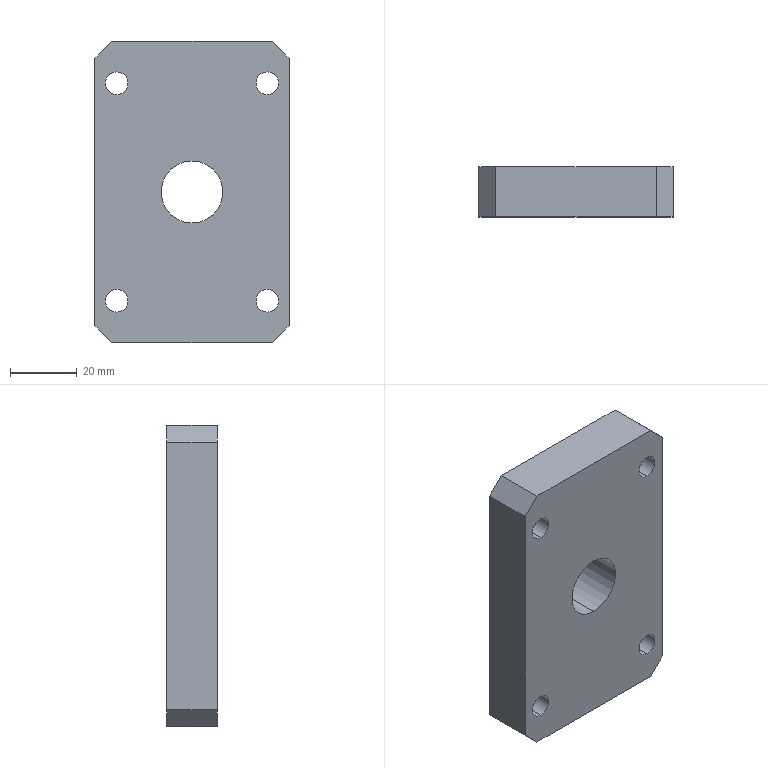Part | SolidWorks | features HoleWzd 2, Chamfer 1, Extrusion 1 | 1 solid | 20 faces | box 58 x 15 x 90 mm | volume 71339 mm3 | cylinder 10 | plane 10 | commonest cylinder face diameters 6.8 x8 18.5 x2
STEP:
#1=CARTESIAN_POINT('',(0.,-7.5,-9.25));
#2=VERTEX_POINT('',#1);
#3=CARTESIAN_POINT('',(0.,-7.5,9.25));
#4=VERTEX_POINT('',#3);
#5=CARTESIAN_POINT('',(0.,-7.5,0.));
#6=DIRECTION('',(0.,1.,0.));
#7=DIRECTION('',(0.,0.,1.));
#8=AXIS2_PLACEMENT_3D('',#5,#6,#7);
#9=CIRCLE('',#8,9.25);
#10=EDGE_CURVE('',#2,#4,#9,.T.);
#11=ORIENTED_EDGE('',*,*,#10,.F.);
#12=CARTESIAN_POINT('',(0.,7.5,-9.25));
#13=VERTEX_POINT('',#12);
#14=CARTESIAN_POINT('',(0.,7.5,-9.25));
#15=DIRECTION('',(0.,1.,0.));
#16=VECTOR('',#15,1000.);
#17=LINE('',#14,#16);
#18=EDGE_CURVE('',#2,#13,#17,.T.);
#19=ORIENTED_EDGE('',*,*,#18,.T.);
#20=CARTESIAN_POINT('',(0.,7.5,9.25));
#21=VERTEX_POINT('',#20);
#22=CARTESIAN_POINT('',(0.,7.5,0.));
#23=DIRECTION('',(0.,1.,0.));
#24=DIRECTION('',(0.,0.,1.));
#25=AXIS2_PLACEMENT_3D('',#22,#23,#24);
#26=CIRCLE('',#25,9.25);
#27=EDGE_CURVE('',#13,#21,#26,.T.);
#28=ORIENTED_EDGE('',*,*,#27,.T.);
#29=CARTESIAN_POINT('',(0.,7.5,9.25));
#30=DIRECTION('',(0.,1.,0.));
#31=VECTOR('',#30,1000.);
#32=LINE('',#29,#31);
#33=EDGE_CURVE('',#4,#21,#32,.T.);
#34=ORIENTED_EDGE('',*,*,#33,.F.);
#35=EDGE_LOOP('',(#11,#19,#28,#34));
#36=FACE_OUTER_BOUND('',#35,.T.);
#37=CARTESIAN_POINT('',(0.,7.5,0.));
#38=DIRECTION('',(0.,1.,0.));
#39=DIRECTION('',(0.,0.,1.));
#40=AXIS2_PLACEMENT_3D('',#37,#38,#39);
#41=CYLINDRICAL_SURFACE('',#40,9.25);
#42=ADVANCED_FACE('',(#36),#41,.F.);
#43=CARTESIAN_POINT('',(-22.5,7.5,-35.9));
#44=VERTEX_POINT('',#43);
#45=CARTESIAN_POINT('',(-22.5,7.5,-29.1));
#46=VERTEX_POINT('',#45);
#47=CARTESIAN_POINT('',(-22.5,7.5,-32.5));
#48=DIRECTION('',(0.,1.,0.));
#49=DIRECTION('',(0.,0.,1.));
#50=AXIS2_PLACEMENT_3D('',#47,#48,#49);
#51=CIRCLE('',#50,3.4);
#52=EDGE_CURVE('',#44,#46,#51,.T.);
#53=ORIENTED_EDGE('',*,*,#52,.T.);
#54=CARTESIAN_POINT('',(-22.5,-7.5,-29.1));
#55=VERTEX_POINT('',#54);
#56=CARTESIAN_POINT('',(-22.5,-7.5,-29.1));
#57=DIRECTION('',(0.,-1.,0.));
#58=VECTOR('',#57,1000.);
#59=LINE('',#56,#58);
#60=EDGE_CURVE('',#46,#55,#59,.T.);
#61=ORIENTED_EDGE('',*,*,#60,.T.);
#62=CARTESIAN_POINT('',(-22.5,-7.5,-35.9));
#63=VERTEX_POINT('',#62);
#64=CARTESIAN_POINT('',(-22.5,-7.5,-32.5));
#65=DIRECTION('',(0.,-1.,0.));
#66=DIRECTION('',(0.,0.,-1.));
#67=AXIS2_PLACEMENT_3D('',#64,#65,#66);
#68=CIRCLE('',#67,3.4);
#69=EDGE_CURVE('',#55,#63,#68,.T.);
#70=ORIENTED_EDGE('',*,*,#69,.T.);
#71=CARTESIAN_POINT('',(-22.5,-7.5,-35.9));
#72=DIRECTION('',(0.,-1.,0.));
#73=VECTOR('',#72,1000.);
#74=LINE('',#71,#73);
#75=EDGE_CURVE('',#44,#63,#74,.T.);
#76=ORIENTED_EDGE('',*,*,#75,.F.);
#77=EDGE_LOOP('',(#53,#61,#70,#76));
#78=FACE_OUTER_BOUND('',#77,.T.);
#79=CARTESIAN_POINT('',(-22.5,-7.5,-32.5));
#80=DIRECTION('',(0.,-1.,0.));
#81=DIRECTION('',(0.,0.,-1.));
#82=AXIS2_PLACEMENT_3D('',#79,#80,#81);
#83=CYLINDRICAL_SURFACE('',#82,3.4);
#84=ADVANCED_FACE('',(#78),#83,.F.);
#85=CARTESIAN_POINT('',(22.5,7.5,-35.9));
#86=VERTEX_POINT('',#85);
#87=CARTESIAN_POINT('',(22.5,7.5,-29.1));
#88=VERTEX_POINT('',#87);
#89=CARTESIAN_POINT('',(22.5,7.5,-32.5));
#90=DIRECTION('',(0.,1.,0.));
#91=DIRECTION('',(0.,0.,1.));
#92=AXIS2_PLACEMENT_3D('',#89,#90,#91);
#93=CIRCLE('',#92,3.4);
#94=EDGE_CURVE('',#86,#88,#93,.T.);
#95=ORIENTED_EDGE('',*,*,#94,.T.);
#96=CARTESIAN_POINT('',(22.5,-7.5,-29.1));
#97=VERTEX_POINT('',#96);
#98=CARTESIAN_POINT('',(22.5,-7.5,-29.1));
#99=DIRECTION('',(0.,-1.,0.));
#100=VECTOR('',#99,1000.);
#101=LINE('',#98,#100);
#102=EDGE_CURVE('',#88,#97,#101,.T.);
#103=ORIENTED_EDGE('',*,*,#102,.T.);
#104=CARTESIAN_POINT('',(22.5,-7.5,-35.9));
#105=VERTEX_POINT('',#104);
#106=CARTESIAN_POINT('',(22.5,-7.5,-32.5));
#107=DIRECTION('',(0.,-1.,0.));
#108=DIRECTION('',(0.,0.,-1.));
#109=AXIS2_PLACEMENT_3D('',#106,#107,#108);
#110=CIRCLE('',#109,3.4);
#111=EDGE_CURVE('',#97,#105,#110,.T.);
#112=ORIENTED_EDGE('',*,*,#111,.T.);
#113=CARTESIAN_POINT('',(22.5,-7.5,-35.9));
#114=DIRECTION('',(0.,-1.,0.));
#115=VECTOR('',#114,1000.);
#116=LINE('',#113,#115);
#117=EDGE_CURVE('',#86,#105,#116,.T.);
#118=ORIENTED_EDGE('',*,*,#117,.F.);
#119=EDGE_LOOP('',(#95,#103,#112,#118));
#120=FACE_OUTER_BOUND('',#119,.T.);
#121=CARTESIAN_POINT('',(22.5,-7.5,-32.5));
#122=DIRECTION('',(0.,-1.,0.));
#123=DIRECTION('',(0.,0.,-1.));
#124=AXIS2_PLACEMENT_3D('',#121,#122,#123);
#125=CYLINDRICAL_SURFACE('',#124,3.4);
#126=ADVANCED_FACE('',(#120),#125,.F.);
#127=CARTESIAN_POINT('',(22.5,7.5,29.1));
#128=VERTEX_POINT('',#127);
#129=CARTESIAN_POINT('',(22.5,7.5,35.9));
#130=VERTEX_POINT('',#129);
#131=CARTESIAN_POINT('',(22.5,7.5,32.5));
#132=DIRECTION('',(0.,1.,0.));
#133=DIRECTION('',(0.,0.,1.));
#134=AXIS2_PLACEMENT_3D('',#131,#132,#133);
#135=CIRCLE('',#134,3.4);
#136=EDGE_CURVE('',#128,#130,#135,.T.);
#137=ORIENTED_EDGE('',*,*,#136,.T.);
#138=CARTESIAN_POINT('',(22.5,-7.5,35.9));
#139=VERTEX_POINT('',#138);
#140=CARTESIAN_POINT('',(22.5,-7.5,35.9));
#141=DIRECTION('',(0.,-1.,0.));
#142=VECTOR('',#141,1000.);
#143=LINE('',#140,#142);
#144=EDGE_CURVE('',#130,#139,#143,.T.);
#145=ORIENTED_EDGE('',*,*,#144,.T.);
#146=CARTESIAN_POINT('',(22.5,-7.5,29.1));
#147=VERTEX_POINT('',#146);
#148=CARTESIAN_POINT('',(22.5,-7.5,32.5));
#149=DIRECTION('',(0.,-1.,0.));
#150=DIRECTION('',(0.,0.,-1.));
#151=AXIS2_PLACEMENT_3D('',#148,#149,#150);
#152=CIRCLE('',#151,3.4);
#153=EDGE_CURVE('',#139,#147,#152,.T.);
#154=ORIENTED_EDGE('',*,*,#153,.T.);
#155=CARTESIAN_POINT('',(22.5,-7.5,29.1));
#156=DIRECTION('',(0.,-1.,0.));
#157=VECTOR('',#156,1000.);
#158=LINE('',#155,#157);
#159=EDGE_CURVE('',#128,#147,#158,.T.);
#160=ORIENTED_EDGE('',*,*,#159,.F.);
#161=EDGE_LOOP('',(#137,#145,#154,#160));
#162=FACE_OUTER_BOUND('',#161,.T.);
#163=CARTESIAN_POINT('',(22.5,-7.5,32.5));
#164=DIRECTION('',(0.,-1.,0.));
#165=DIRECTION('',(0.,0.,-1.));
#166=AXIS2_PLACEMENT_3D('',#163,#164,#165);
#167=CYLINDRICAL_SURFACE('',#166,3.4);
#168=ADVANCED_FACE('',(#162),#167,.F.);
#169=CARTESIAN_POINT('',(-22.5,7.5,29.1));
#170=VERTEX_POINT('',#169);
#171=CARTESIAN_POINT('',(-22.5,7.5,35.9));
#172=VERTEX_POINT('',#171);
#173=CARTESIAN_POINT('',(-22.5,7.5,32.5));
#174=DIRECTION('',(0.,1.,0.));
#175=DIRECTION('',(0.,0.,1.));
#176=AXIS2_PLACEMENT_3D('',#173,#174,#175);
#177=CIRCLE('',#176,3.4);
#178=EDGE_CURVE('',#170,#172,#177,.T.);
#179=ORIENTED_EDGE('',*,*,#178,.T.);
#180=CARTESIAN_POINT('',(-22.5,-7.5,35.9));
#181=VERTEX_POINT('',#180);
#182=CARTESIAN_POINT('',(-22.5,-7.5,35.9));
#183=DIRECTION('',(0.,-1.,0.));
#184=VECTOR('',#183,1000.);
#185=LINE('',#182,#184);
#186=EDGE_CURVE('',#172,#181,#185,.T.);
#187=ORIENTED_EDGE('',*,*,#186,.T.);
#188=CARTESIAN_POINT('',(-22.5,-7.5,29.1));
#189=VERTEX_POINT('',#188);
#190=CARTESIAN_POINT('',(-22.5,-7.5,32.5));
#191=DIRECTION('',(0.,-1.,0.));
#192=DIRECTION('',(0.,0.,-1.));
#193=AXIS2_PLACEMENT_3D('',#190,#191,#192);
#194=CIRCLE('',#193,3.4);
#195=EDGE_CURVE('',#181,#189,#194,.T.);
#196=ORIENTED_EDGE('',*,*,#195,.T.);
#197=CARTESIAN_POINT('',(-22.5,-7.5,29.1));
#198=DIRECTION('',(0.,-1.,0.));
#199=VECTOR('',#198,1000.);
#200=LINE('',#197,#199);
#201=EDGE_CURVE('',#170,#189,#200,.T.);
#202=ORIENTED_EDGE('',*,*,#201,.F.);
#203=EDGE_LOOP('',(#179,#187,#196,#202));
#204=FACE_OUTER_BOUND('',#203,.T.);
#205=CARTESIAN_POINT('',(-22.5,-7.5,32.5));
#206=DIRECTION('',(0.,-1.,0.));
#207=DIRECTION('',(0.,0.,-1.));
#208=AXIS2_PLACEMENT_3D('',#205,#206,#207);
#209=CYLINDRICAL_SURFACE('',#208,3.4);
#210=ADVANCED_FACE('',(#204),#209,.F.);
#211=CARTESIAN_POINT('',(29.,7.5,40.));
#212=VERTEX_POINT('',#211);
#213=CARTESIAN_POINT('',(29.,7.5,-40.));
#214=VERTEX_POINT('',#213);
#215=CARTESIAN_POINT('',(29.,7.5,-45.));
#216=DIRECTION('',(0.,0.,-1.));
#217=VECTOR('',#216,1000.);
#218=LINE('',#215,#217);
#219=EDGE_CURVE('',#212,#214,#218,.T.);
#220=ORIENTED_EDGE('',*,*,#219,.F.);
#221=CARTESIAN_POINT('',(29.,-7.5,40.));
#222=VERTEX_POINT('',#221);
#223=CARTESIAN_POINT('',(29.,7.5,40.));
#224=DIRECTION('',(0.,-1.,0.));
#225=VECTOR('',#224,1000.);
#226=LINE('',#223,#225);
#227=EDGE_CURVE('',#212,#222,#226,.T.);
#228=ORIENTED_EDGE('',*,*,#227,.T.);
#229=CARTESIAN_POINT('',(29.,-7.5,-40.));
#230=VERTEX_POINT('',#229);
#231=CARTESIAN_POINT('',(29.,-7.5,-45.));
#232=DIRECTION('',(0.,0.,-1.));
#233=VECTOR('',#232,1000.);
#234=LINE('',#231,#233);
#235=EDGE_CURVE('',#222,#230,#234,.T.);
#236=ORIENTED_EDGE('',*,*,#235,.T.);
#237=CARTESIAN_POINT('',(29.,7.5,-40.));
#238=DIRECTION('',(0.,1.,0.));
#239=VECTOR('',#238,1000.);
#240=LINE('',#237,#239);
#241=EDGE_CURVE('',#230,#214,#240,.T.);
#242=ORIENTED_EDGE('',*,*,#241,.T.);
#243=EDGE_LOOP('',(#220,#228,#236,#242));
#244=FACE_OUTER_BOUND('',#243,.T.);
#245=CARTESIAN_POINT('',(29.,7.5,-45.));
#246=DIRECTION('',(-1.,0.,0.));
#247=DIRECTION('',(0.,0.,1.));
#248=AXIS2_PLACEMENT_3D('',#245,#246,#247);
#249=PLANE('',#248);
#250=ADVANCED_FACE('',(#244),#249,.F.);
#251=CARTESIAN_POINT('',(24.,7.5,-45.));
#252=VERTEX_POINT('',#251);
#253=CARTESIAN_POINT('',(-24.,7.5,-45.));
#254=VERTEX_POINT('',#253);
#255=CARTESIAN_POINT('',(-29.,7.5,-45.));
#256=DIRECTION('',(-1.,0.,0.));
#257=VECTOR('',#256,1000.);
#258=LINE('',#255,#257);
#259=EDGE_CURVE('',#252,#254,#258,.T.);
#260=ORIENTED_EDGE('',*,*,#259,.F.);
#261=CARTESIAN_POINT('',(24.,-7.5,-45.));
#262=VERTEX_POINT('',#261);
#263=CARTESIAN_POINT('',(24.,7.5,-45.));
#264=DIRECTION('',(0.,-1.,0.));
#265=VECTOR('',#264,1000.);
#266=LINE('',#263,#265);
#267=EDGE_CURVE('',#252,#262,#266,.T.);
#268=ORIENTED_EDGE('',*,*,#267,.T.);
#269=CARTESIAN_POINT('',(-24.,-7.5,-45.));
#270=VERTEX_POINT('',#269);
#271=CARTESIAN_POINT('',(-29.,-7.5,-45.));
#272=DIRECTION('',(-1.,0.,0.));
#273=VECTOR('',#272,1000.);
#274=LINE('',#271,#273);
#275=EDGE_CURVE('',#262,#270,#274,.T.);
#276=ORIENTED_EDGE('',*,*,#275,.T.);
#277=CARTESIAN_POINT('',(-24.,7.5,-45.));
#278=DIRECTION('',(0.,1.,0.));
#279=VECTOR('',#278,1000.);
#280=LINE('',#277,#279);
#281=EDGE_CURVE('',#270,#254,#280,.T.);
#282=ORIENTED_EDGE('',*,*,#281,.T.);
#283=EDGE_LOOP('',(#260,#268,#276,#282));
#284=FACE_OUTER_BOUND('',#283,.T.);
#285=CARTESIAN_POINT('',(-29.,7.5,-45.));
#286=DIRECTION('',(0.,0.,1.));
#287=DIRECTION('',(1.,0.,0.));
#288=AXIS2_PLACEMENT_3D('',#285,#286,#287);
#289=PLANE('',#288);
#290=ADVANCED_FACE('',(#284),#289,.F.);
#291=CARTESIAN_POINT('',(-29.,7.5,-40.));
#292=VERTEX_POINT('',#291);
#293=CARTESIAN_POINT('',(-29.,7.5,40.));
#294=VERTEX_POINT('',#293);
#295=CARTESIAN_POINT('',(-29.,7.5,-45.));
#296=DIRECTION('',(0.,0.,1.));
#297=VECTOR('',#296,1000.);
#298=LINE('',#295,#297);
#299=EDGE_CURVE('',#292,#294,#298,.T.);
#300=ORIENTED_EDGE('',*,*,#299,.F.);
#301=CARTESIAN_POINT('',(-29.,-7.5,-40.));
#302=VERTEX_POINT('',#301);
#303=CARTESIAN_POINT('',(-29.,7.5,-40.));
#304=DIRECTION('',(0.,-1.,0.));
#305=VECTOR('',#304,1000.);
#306=LINE('',#303,#305);
#307=EDGE_CURVE('',#292,#302,#306,.T.);
#308=ORIENTED_EDGE('',*,*,#307,.T.);
#309=CARTESIAN_POINT('',(-29.,-7.5,40.));
#310=VERTEX_POINT('',#309);
#311=CARTESIAN_POINT('',(-29.,-7.5,-45.));
#312=DIRECTION('',(0.,0.,1.));
#313=VECTOR('',#312,1000.);
#314=LINE('',#311,#313);
#315=EDGE_CURVE('',#302,#310,#314,.T.);
#316=ORIENTED_EDGE('',*,*,#315,.T.);
#317=CARTESIAN_POINT('',(-29.,7.5,40.));
#318=DIRECTION('',(0.,1.,0.));
#319=VECTOR('',#318,1000.);
#320=LINE('',#317,#319);
#321=EDGE_CURVE('',#310,#294,#320,.T.);
#322=ORIENTED_EDGE('',*,*,#321,.T.);
#323=EDGE_LOOP('',(#300,#308,#316,#322));
#324=FACE_OUTER_BOUND('',#323,.T.);
#325=CARTESIAN_POINT('',(-29.,7.5,-45.));
#326=DIRECTION('',(1.,0.,0.));
#327=DIRECTION('',(0.,0.,-1.));
#328=AXIS2_PLACEMENT_3D('',#325,#326,#327);
#329=PLANE('',#328);
#330=ADVANCED_FACE('',(#324),#329,.F.);
#331=CARTESIAN_POINT('',(-24.,-7.5,45.));
#332=VERTEX_POINT('',#331);
#333=CARTESIAN_POINT('',(24.,-7.5,45.));
#334=VERTEX_POINT('',#333);
#335=CARTESIAN_POINT('',(-29.,-7.5,45.));
#336=DIRECTION('',(1.,0.,0.));
#337=VECTOR('',#336,1000.);
#338=LINE('',#335,#337);
#339=EDGE_CURVE('',#332,#334,#338,.T.);
#340=ORIENTED_EDGE('',*,*,#339,.T.);
#341=CARTESIAN_POINT('',(24.,7.5,45.));
#342=VERTEX_POINT('',#341);
#343=CARTESIAN_POINT('',(24.,7.5,45.));
#344=DIRECTION('',(0.,1.,0.));
#345=VECTOR('',#344,1000.);
#346=LINE('',#343,#345);
#347=EDGE_CURVE('',#334,#342,#346,.T.);
#348=ORIENTED_EDGE('',*,*,#347,.T.);
#349=CARTESIAN_POINT('',(-24.,7.5,45.));
#350=VERTEX_POINT('',#349);
#351=CARTESIAN_POINT('',(-29.,7.5,45.));
#352=DIRECTION('',(1.,0.,0.));
#353=VECTOR('',#352,1000.);
#354=LINE('',#351,#353);
#355=EDGE_CURVE('',#350,#342,#354,.T.);
#356=ORIENTED_EDGE('',*,*,#355,.F.);
#357=CARTESIAN_POINT('',(-24.,7.5,45.));
#358=DIRECTION('',(0.,-1.,0.));
#359=VECTOR('',#358,1000.);
#360=LINE('',#357,#359);
#361=EDGE_CURVE('',#350,#332,#360,.T.);
#362=ORIENTED_EDGE('',*,*,#361,.T.);
#363=EDGE_LOOP('',(#340,#348,#356,#362));
#364=FACE_OUTER_BOUND('',#363,.T.);
#365=CARTESIAN_POINT('',(-29.,7.5,45.));
#366=DIRECTION('',(0.,0.,-1.));
#367=DIRECTION('',(-1.,0.,0.));
#368=AXIS2_PLACEMENT_3D('',#365,#366,#367);
#369=PLANE('',#368);
#370=ADVANCED_FACE('',(#364),#369,.F.);
#371=CARTESIAN_POINT('',(0.,7.5,0.));
#372=DIRECTION('',(0.,1.,0.));
#373=DIRECTION('',(0.,0.,1.));
#374=AXIS2_PLACEMENT_3D('',#371,#372,#373);
#375=CIRCLE('',#374,9.25);
#376=EDGE_CURVE('',#21,#13,#375,.T.);
#377=ORIENTED_EDGE('',*,*,#376,.F.);
#378=ORIENTED_EDGE('',*,*,#27,.F.);
#379=EDGE_LOOP('',(#377,#378));
#380=FACE_BOUND('',#379,.T.);
#381=ORIENTED_EDGE('',*,*,#52,.F.);
#382=CARTESIAN_POINT('',(-22.5,7.5,-32.5));
#383=DIRECTION('',(0.,1.,0.));
#384=DIRECTION('',(0.,0.,1.));
#385=AXIS2_PLACEMENT_3D('',#382,#383,#384);
#386=CIRCLE('',#385,3.4);
#387=EDGE_CURVE('',#46,#44,#386,.T.);
#388=ORIENTED_EDGE('',*,*,#387,.F.);
#389=EDGE_LOOP('',(#381,#388));
#390=FACE_BOUND('',#389,.T.);
#391=ORIENTED_EDGE('',*,*,#94,.F.);
#392=CARTESIAN_POINT('',(22.5,7.5,-32.5));
#393=DIRECTION('',(0.,1.,0.));
#394=DIRECTION('',(0.,0.,1.));
#395=AXIS2_PLACEMENT_3D('',#392,#393,#394);
#396=CIRCLE('',#395,3.4);
#397=EDGE_CURVE('',#88,#86,#396,.T.);
#398=ORIENTED_EDGE('',*,*,#397,.F.);
#399=EDGE_LOOP('',(#391,#398));
#400=FACE_BOUND('',#399,.T.);
#401=ORIENTED_EDGE('',*,*,#136,.F.);
#402=CARTESIAN_POINT('',(22.5,7.5,32.5));
#403=DIRECTION('',(0.,1.,0.));
#404=DIRECTION('',(0.,0.,1.));
#405=AXIS2_PLACEMENT_3D('',#402,#403,#404);
#406=CIRCLE('',#405,3.4);
#407=EDGE_CURVE('',#130,#128,#406,.T.);
#408=ORIENTED_EDGE('',*,*,#407,.F.);
#409=EDGE_LOOP('',(#401,#408));
#410=FACE_BOUND('',#409,.T.);
#411=ORIENTED_EDGE('',*,*,#178,.F.);
#412=CARTESIAN_POINT('',(-22.5,7.5,32.5));
#413=DIRECTION('',(0.,1.,0.));
#414=DIRECTION('',(0.,0.,1.));
#415=AXIS2_PLACEMENT_3D('',#412,#413,#414);
#416=CIRCLE('',#415,3.4);
#417=EDGE_CURVE('',#172,#170,#416,.T.);
#418=ORIENTED_EDGE('',*,*,#417,.F.);
#419=EDGE_LOOP('',(#411,#418));
#420=FACE_BOUND('',#419,.T.);
#421=ORIENTED_EDGE('',*,*,#355,.T.);
#422=CARTESIAN_POINT('',(34.5,7.5,34.5));
#423=DIRECTION('',(0.7071,0.,-0.7071));
#424=VECTOR('',#423,1000.);
#425=LINE('',#422,#424);
#426=EDGE_CURVE('',#342,#212,#425,.T.);
#427=ORIENTED_EDGE('',*,*,#426,.T.);
#428=ORIENTED_EDGE('',*,*,#219,.T.);
#429=CARTESIAN_POINT('',(34.5,7.5,-34.5));
#430=DIRECTION('',(-0.7071,0.,-0.7071));
#431=VECTOR('',#430,1000.);
#432=LINE('',#429,#431);
#433=EDGE_CURVE('',#214,#252,#432,.T.);
#434=ORIENTED_EDGE('',*,*,#433,.T.);
#435=ORIENTED_EDGE('',*,*,#259,.T.);
#436=CARTESIAN_POINT('',(-34.5,7.5,-34.5));
#437=DIRECTION('',(-0.7071,0.,0.7071));
#438=VECTOR('',#437,1000.);
#439=LINE('',#436,#438);
#440=EDGE_CURVE('',#254,#292,#439,.T.);
#441=ORIENTED_EDGE('',*,*,#440,.T.);
#442=ORIENTED_EDGE('',*,*,#299,.T.);
#443=CARTESIAN_POINT('',(-34.5,7.5,34.5));
#444=DIRECTION('',(0.7071,0.,0.7071));
#445=VECTOR('',#444,1000.);
#446=LINE('',#443,#445);
#447=EDGE_CURVE('',#294,#350,#446,.T.);
#448=ORIENTED_EDGE('',*,*,#447,.T.);
#449=EDGE_LOOP('',(#421,#427,#428,#434,#435,#441,#442,#448));
#450=FACE_OUTER_BOUND('',#449,.T.);
#451=CARTESIAN_POINT('',(0.,7.5,0.));
#452=DIRECTION('',(0.,1.,0.));
#453=DIRECTION('',(0.,0.,1.));
#454=AXIS2_PLACEMENT_3D('',#451,#452,#453);
#455=PLANE('',#454);
#456=ADVANCED_FACE('',(#380,#390,#400,#410,#420,#450),#455,.T.);
#457=CARTESIAN_POINT('',(0.,-7.5,0.));
#458=DIRECTION('',(0.,1.,0.));
#459=DIRECTION('',(0.,0.,1.));
#460=AXIS2_PLACEMENT_3D('',#457,#458,#459);
#461=CIRCLE('',#460,9.25);
#462=EDGE_CURVE('',#4,#2,#461,.T.);
#463=ORIENTED_EDGE('',*,*,#462,.T.);
#464=ORIENTED_EDGE('',*,*,#10,.T.);
#465=EDGE_LOOP('',(#463,#464));
#466=FACE_BOUND('',#465,.T.);
#467=CARTESIAN_POINT('',(-22.5,-7.5,-32.5));
#468=DIRECTION('',(0.,-1.,0.));
#469=DIRECTION('',(0.,0.,-1.));
#470=AXIS2_PLACEMENT_3D('',#467,#468,#469);
#471=CIRCLE('',#470,3.4);
#472=EDGE_CURVE('',#63,#55,#471,.T.);
#473=ORIENTED_EDGE('',*,*,#472,.F.);
#474=ORIENTED_EDGE('',*,*,#69,.F.);
#475=EDGE_LOOP('',(#473,#474));
#476=FACE_BOUND('',#475,.T.);
#477=CARTESIAN_POINT('',(22.5,-7.5,-32.5));
#478=DIRECTION('',(0.,-1.,0.));
#479=DIRECTION('',(0.,0.,-1.));
#480=AXIS2_PLACEMENT_3D('',#477,#478,#479);
#481=CIRCLE('',#480,3.4);
#482=EDGE_CURVE('',#105,#97,#481,.T.);
#483=ORIENTED_EDGE('',*,*,#482,.F.);
#484=ORIENTED_EDGE('',*,*,#111,.F.);
#485=EDGE_LOOP('',(#483,#484));
#486=FACE_BOUND('',#485,.T.);
#487=CARTESIAN_POINT('',(22.5,-7.5,32.5));
#488=DIRECTION('',(0.,-1.,0.));
#489=DIRECTION('',(0.,0.,-1.));
#490=AXIS2_PLACEMENT_3D('',#487,#488,#489);
#491=CIRCLE('',#490,3.4);
#492=EDGE_CURVE('',#147,#139,#491,.T.);
#493=ORIENTED_EDGE('',*,*,#492,.F.);
#494=ORIENTED_EDGE('',*,*,#153,.F.);
#495=EDGE_LOOP('',(#493,#494));
#496=FACE_BOUND('',#495,.T.);
#497=CARTESIAN_POINT('',(-22.5,-7.5,32.5));
#498=DIRECTION('',(0.,-1.,0.));
#499=DIRECTION('',(0.,0.,-1.));
#500=AXIS2_PLACEMENT_3D('',#497,#498,#499);
#501=CIRCLE('',#500,3.4);
#502=EDGE_CURVE('',#189,#181,#501,.T.);
#503=ORIENTED_EDGE('',*,*,#502,.F.);
#504=ORIENTED_EDGE('',*,*,#195,.F.);
#505=EDGE_LOOP('',(#503,#504));
#506=FACE_BOUND('',#505,.T.);
#507=ORIENTED_EDGE('',*,*,#235,.F.);
#508=CARTESIAN_POINT('',(29.,-7.5,40.));
#509=DIRECTION('',(-0.7071,0.,0.7071));
#510=VECTOR('',#509,1000.);
#511=LINE('',#508,#510);
#512=EDGE_CURVE('',#222,#334,#511,.T.);
#513=ORIENTED_EDGE('',*,*,#512,.T.);
#514=ORIENTED_EDGE('',*,*,#339,.F.);
#515=CARTESIAN_POINT('',(-24.,-7.5,45.));
#516=DIRECTION('',(-0.7071,0.,-0.7071));
#517=VECTOR('',#516,1000.);
#518=LINE('',#515,#517);
#519=EDGE_CURVE('',#332,#310,#518,.T.);
#520=ORIENTED_EDGE('',*,*,#519,.T.);
#521=ORIENTED_EDGE('',*,*,#315,.F.);
#522=CARTESIAN_POINT('',(-29.,-7.5,-40.));
#523=DIRECTION('',(0.7071,0.,-0.7071));
#524=VECTOR('',#523,1000.);
#525=LINE('',#522,#524);
#526=EDGE_CURVE('',#302,#270,#525,.T.);
#527=ORIENTED_EDGE('',*,*,#526,.T.);
#528=ORIENTED_EDGE('',*,*,#275,.F.);
#529=CARTESIAN_POINT('',(24.,-7.5,-45.));
#530=DIRECTION('',(0.7071,0.,0.7071));
#531=VECTOR('',#530,1000.);
#532=LINE('',#529,#531);
#533=EDGE_CURVE('',#262,#230,#532,.T.);
#534=ORIENTED_EDGE('',*,*,#533,.T.);
#535=EDGE_LOOP('',(#507,#513,#514,#520,#521,#527,#528,#534));
#536=FACE_OUTER_BOUND('',#535,.T.);
#537=CARTESIAN_POINT('',(0.,-7.5,0.));
#538=DIRECTION('',(0.,1.,0.));
#539=DIRECTION('',(0.,0.,1.));
#540=AXIS2_PLACEMENT_3D('',#537,#538,#539);
#541=PLANE('',#540);
#542=ADVANCED_FACE('',(#466,#476,#486,#496,#506,#536),#541,.F.);
#543=ORIENTED_EDGE('',*,*,#186,.F.);
#544=ORIENTED_EDGE('',*,*,#417,.T.);
#545=ORIENTED_EDGE('',*,*,#201,.T.);
#546=ORIENTED_EDGE('',*,*,#502,.T.);
#547=EDGE_LOOP('',(#543,#544,#545,#546));
#548=FACE_OUTER_BOUND('',#547,.T.);
#549=CARTESIAN_POINT('',(-22.5,-7.5,32.5));
#550=DIRECTION('',(0.,-1.,0.));
#551=DIRECTION('',(0.,0.,-1.));
#552=AXIS2_PLACEMENT_3D('',#549,#550,#551);
#553=CYLINDRICAL_SURFACE('',#552,3.4);
#554=ADVANCED_FACE('',(#548),#553,.F.);
#555=ORIENTED_EDGE('',*,*,#144,.F.);
#556=ORIENTED_EDGE('',*,*,#407,.T.);
#557=ORIENTED_EDGE('',*,*,#159,.T.);
#558=ORIENTED_EDGE('',*,*,#492,.T.);
#559=EDGE_LOOP('',(#555,#556,#557,#558));
#560=FACE_OUTER_BOUND('',#559,.T.);
#561=CARTESIAN_POINT('',(22.5,-7.5,32.5));
#562=DIRECTION('',(0.,-1.,0.));
#563=DIRECTION('',(0.,0.,-1.));
#564=AXIS2_PLACEMENT_3D('',#561,#562,#563);
#565=CYLINDRICAL_SURFACE('',#564,3.4);
#566=ADVANCED_FACE('',(#560),#565,.F.);
#567=ORIENTED_EDGE('',*,*,#102,.F.);
#568=ORIENTED_EDGE('',*,*,#397,.T.);
#569=ORIENTED_EDGE('',*,*,#117,.T.);
#570=ORIENTED_EDGE('',*,*,#482,.T.);
#571=EDGE_LOOP('',(#567,#568,#569,#570));
#572=FACE_OUTER_BOUND('',#571,.T.);
#573=CARTESIAN_POINT('',(22.5,-7.5,-32.5));
#574=DIRECTION('',(0.,-1.,0.));
#575=DIRECTION('',(0.,0.,-1.));
#576=AXIS2_PLACEMENT_3D('',#573,#574,#575);
#577=CYLINDRICAL_SURFACE('',#576,3.4);
#578=ADVANCED_FACE('',(#572),#577,.F.);
#579=ORIENTED_EDGE('',*,*,#60,.F.);
#580=ORIENTED_EDGE('',*,*,#387,.T.);
#581=ORIENTED_EDGE('',*,*,#75,.T.);
#582=ORIENTED_EDGE('',*,*,#472,.T.);
#583=EDGE_LOOP('',(#579,#580,#581,#582));
#584=FACE_OUTER_BOUND('',#583,.T.);
#585=CARTESIAN_POINT('',(-22.5,-7.5,-32.5));
#586=DIRECTION('',(0.,-1.,0.));
#587=DIRECTION('',(0.,0.,-1.));
#588=AXIS2_PLACEMENT_3D('',#585,#586,#587);
#589=CYLINDRICAL_SURFACE('',#588,3.4);
#590=ADVANCED_FACE('',(#584),#589,.F.);
#591=ORIENTED_EDGE('',*,*,#18,.F.);
#592=ORIENTED_EDGE('',*,*,#462,.F.);
#593=ORIENTED_EDGE('',*,*,#33,.T.);
#594=ORIENTED_EDGE('',*,*,#376,.T.);
#595=EDGE_LOOP('',(#591,#592,#593,#594));
#596=FACE_OUTER_BOUND('',#595,.T.);
#597=CARTESIAN_POINT('',(0.,7.5,0.));
#598=DIRECTION('',(0.,1.,0.));
#599=DIRECTION('',(0.,0.,1.));
#600=AXIS2_PLACEMENT_3D('',#597,#598,#599);
#601=CYLINDRICAL_SURFACE('',#600,9.25);
#602=ADVANCED_FACE('',(#596),#601,.F.);
#603=ORIENTED_EDGE('',*,*,#426,.F.);
#604=ORIENTED_EDGE('',*,*,#347,.F.);
#605=ORIENTED_EDGE('',*,*,#512,.F.);
#606=ORIENTED_EDGE('',*,*,#227,.F.);
#607=EDGE_LOOP('',(#603,#604,#605,#606));
#608=FACE_OUTER_BOUND('',#607,.T.);
#609=CARTESIAN_POINT('',(29.,7.5,40.));
#610=DIRECTION('',(-0.7071,0.,-0.7071));
#611=DIRECTION('',(0.,-1.,0.));
#612=AXIS2_PLACEMENT_3D('',#609,#610,#611);
#613=PLANE('',#612);
#614=ADVANCED_FACE('',(#608),#613,.F.);
#615=ORIENTED_EDGE('',*,*,#433,.F.);
#616=ORIENTED_EDGE('',*,*,#241,.F.);
#617=ORIENTED_EDGE('',*,*,#533,.F.);
#618=ORIENTED_EDGE('',*,*,#267,.F.);
#619=EDGE_LOOP('',(#615,#616,#617,#618));
#620=FACE_OUTER_BOUND('',#619,.T.);
#621=CARTESIAN_POINT('',(24.,7.5,-45.));
#622=DIRECTION('',(-0.7071,0.,0.7071));
#623=DIRECTION('',(0.,-1.,0.));
#624=AXIS2_PLACEMENT_3D('',#621,#622,#623);
#625=PLANE('',#624);
#626=ADVANCED_FACE('',(#620),#625,.F.);
#627=ORIENTED_EDGE('',*,*,#440,.F.);
#628=ORIENTED_EDGE('',*,*,#281,.F.);
#629=ORIENTED_EDGE('',*,*,#526,.F.);
#630=ORIENTED_EDGE('',*,*,#307,.F.);
#631=EDGE_LOOP('',(#627,#628,#629,#630));
#632=FACE_OUTER_BOUND('',#631,.T.);
#633=CARTESIAN_POINT('',(-29.,7.5,-40.));
#634=DIRECTION('',(0.7071,0.,0.7071));
#635=DIRECTION('',(0.,-1.,0.));
#636=AXIS2_PLACEMENT_3D('',#633,#634,#635);
#637=PLANE('',#636);
#638=ADVANCED_FACE('',(#632),#637,.F.);
#639=ORIENTED_EDGE('',*,*,#447,.F.);
#640=ORIENTED_EDGE('',*,*,#321,.F.);
#641=ORIENTED_EDGE('',*,*,#519,.F.);
#642=ORIENTED_EDGE('',*,*,#361,.F.);
#643=EDGE_LOOP('',(#639,#640,#641,#642));
#644=FACE_OUTER_BOUND('',#643,.T.);
#645=CARTESIAN_POINT('',(-24.,7.5,45.));
#646=DIRECTION('',(0.7071,0.,-0.7071));
#647=DIRECTION('',(0.,-1.,0.));
#648=AXIS2_PLACEMENT_3D('',#645,#646,#647);
#649=PLANE('',#648);
#650=ADVANCED_FACE('',(#644),#649,.F.);
#651=CLOSED_SHELL('',(#42,#84,#126,#168,#210,#250,#290,#330,#370,#456,#542,#554,#566,#578,#590,#602,#614,#626,#638,#650));
#652=MANIFOLD_SOLID_BREP('',#651);
#653=CARTESIAN_POINT('',(0.,0.,0.));
#654=DIRECTION('',(0.,0.,1.));
#655=DIRECTION('',(1.,0.,0.));
#656=AXIS2_PLACEMENT_3D('',#653,#654,#655);
#657=(LENGTH_UNIT()NAMED_UNIT(*)SI_UNIT(.MILLI.,.METRE.));
#658=UNCERTAINTY_MEASURE_WITH_UNIT(LENGTH_MEASURE(0.00001),#657,'','');
#659=(NAMED_UNIT(*)PLANE_ANGLE_UNIT()SI_UNIT($,.RADIAN.));
#660=(NAMED_UNIT(*)SI_UNIT($,.STERADIAN.)SOLID_ANGLE_UNIT());
#661=(GEOMETRIC_REPRESENTATION_CONTEXT(3)GLOBAL_UNCERTAINTY_ASSIGNED_CONTEXT((#658))GLOBAL_UNIT_ASSIGNED_CONTEXT((#657,#659,#660))REPRESENTATION_CONTEXT('',''));
#662=ADVANCED_BREP_SHAPE_REPRESENTATION('',(#652,#656),#661);